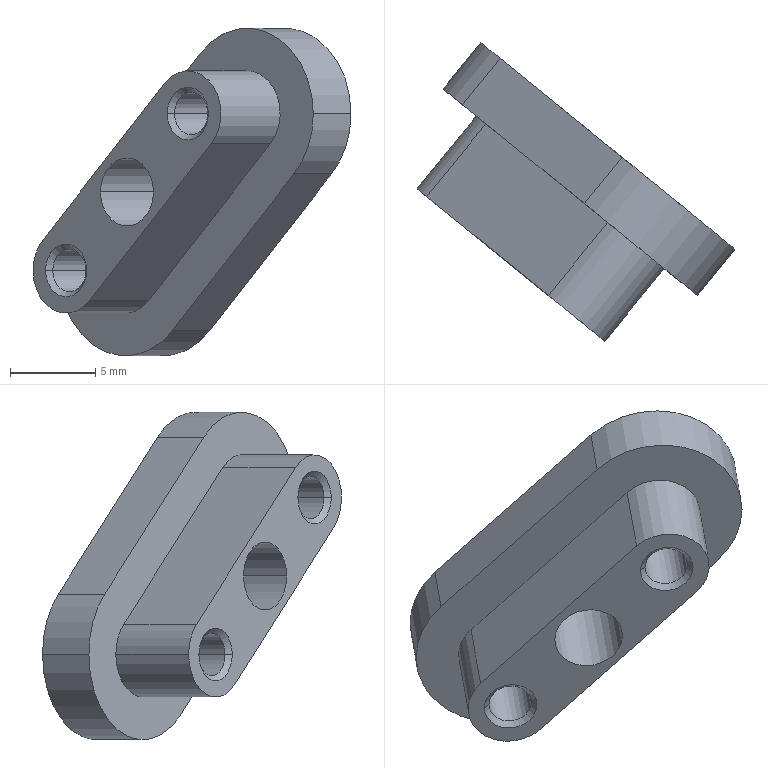Part | SolidWorks | features BaseBody 1 | 1 solid | 28 faces | box 18.629 x 17.514 x 19.192 mm | volume 992.4 mm3 | cylinder 13 | cone 8 | plane 7 | commonest cylinder face diameters 2.5 x4 10 x4 5 x3 4 x2
STEP:
#1=CARTESIAN_POINT('',(538.653,-159.567,279.158));
#2=VERTEX_POINT('',#1);
#3=CARTESIAN_POINT('',(536.714,-157.99,279.158));
#4=VERTEX_POINT('',#3);
#5=CARTESIAN_POINT('',(537.683,-158.779,279.158));
#6=DIRECTION('',(0.6309,0.7758,-0.000000012));
#7=DIRECTION('',(0.5486,-0.4461,0.7071));
#8=AXIS2_PLACEMENT_3D('',#5,#6,#7);
#9=CIRCLE('',#8,1.25);
#10=EDGE_CURVE('',#2,#4,#9,.T.);
#11=ORIENTED_EDGE('',*,*,#10,.F.);
#12=CARTESIAN_POINT('',(539.075,-159.524,279.158));
#13=VERTEX_POINT('',#12);
#14=CARTESIAN_POINT('',(539.075,-159.524,279.158));
#15=DIRECTION('',(0.9947,0.1025,-0.000000009));
#16=VECTOR('',#15,1000.);
#17=LINE('',#14,#16);
#18=EDGE_CURVE('',#2,#13,#17,.T.);
#19=ORIENTED_EDGE('',*,*,#18,.T.);
#20=CARTESIAN_POINT('',(536.67,-157.568,279.158));
#21=VERTEX_POINT('',#20);
#22=CARTESIAN_POINT('',(537.873,-158.546,279.158));
#23=DIRECTION('',(-0.6309,-0.7758,0.000000012));
#24=DIRECTION('',(-0.7758,0.6309,0.));
#25=AXIS2_PLACEMENT_3D('',#22,#23,#24);
#26=CIRCLE('',#25,1.55);
#27=EDGE_CURVE('',#21,#13,#26,.T.);
#28=ORIENTED_EDGE('',*,*,#27,.F.);
#29=CARTESIAN_POINT('',(536.67,-157.568,279.158));
#30=DIRECTION('',(-0.1025,0.9947,-0.000000009));
#31=VECTOR('',#30,1000.);
#32=LINE('',#29,#31);
#33=EDGE_CURVE('',#4,#21,#32,.T.);
#34=ORIENTED_EDGE('',*,*,#33,.F.);
#35=EDGE_LOOP('',(#11,#19,#28,#34));
#36=FACE_OUTER_BOUND('',#35,.T.);
#37=CARTESIAN_POINT('',(537.873,-158.546,279.158));
#38=DIRECTION('',(0.6309,0.7758,-0.000000012));
#39=DIRECTION('',(-0.7758,0.6309,0.));
#40=AXIS2_PLACEMENT_3D('',#37,#38,#39);
#41=CONICAL_SURFACE('',#40,1.55,0.7854);
#42=ADVANCED_FACE('',(#36),#41,.F.);
#43=CARTESIAN_POINT('',(541.752,-161.7,279.158));
#44=VERTEX_POINT('',#43);
#45=CARTESIAN_POINT('',(540.616,-160.776,275.623));
#46=VERTEX_POINT('',#45);
#47=CARTESIAN_POINT('',(537.873,-158.546,279.158));
#48=DIRECTION('',(0.6309,0.7758,-0.000000012));
#49=DIRECTION('',(0.7758,-0.6309,0.));
#50=AXIS2_PLACEMENT_3D('',#47,#48,#49);
#51=CIRCLE('',#50,5.);
#52=EDGE_CURVE('',#44,#46,#51,.T.);
#53=ORIENTED_EDGE('',*,*,#52,.F.);
#54=CARTESIAN_POINT('',(539.544,-164.416,279.158));
#55=VERTEX_POINT('',#54);
#56=CARTESIAN_POINT('',(537.493,-166.937,279.158));
#57=DIRECTION('',(-0.6309,-0.7758,0.000000012));
#58=VECTOR('',#57,1000.);
#59=LINE('',#56,#58);
#60=EDGE_CURVE('',#44,#55,#59,.T.);
#61=ORIENTED_EDGE('',*,*,#60,.T.);
#62=CARTESIAN_POINT('',(538.407,-163.492,275.623));
#63=VERTEX_POINT('',#62);
#64=CARTESIAN_POINT('',(535.664,-161.261,279.158));
#65=DIRECTION('',(0.6309,0.7758,-0.000000012));
#66=DIRECTION('',(0.7758,-0.6309,0.));
#67=AXIS2_PLACEMENT_3D('',#64,#65,#66);
#68=CIRCLE('',#67,5.);
#69=EDGE_CURVE('',#55,#63,#68,.T.);
#70=ORIENTED_EDGE('',*,*,#69,.T.);
#71=CARTESIAN_POINT('',(540.616,-160.776,275.623));
#72=DIRECTION('',(-0.6309,-0.7758,0.000000012));
#73=VECTOR('',#72,1000.);
#74=LINE('',#71,#73);
#75=EDGE_CURVE('',#46,#63,#74,.T.);
#76=ORIENTED_EDGE('',*,*,#75,.F.);
#77=EDGE_LOOP('',(#53,#61,#70,#76));
#78=FACE_OUTER_BOUND('',#77,.T.);
#79=CARTESIAN_POINT('',(533.614,-163.783,279.158));
#80=DIRECTION('',(-0.6309,-0.7758,0.000000012));
#81=DIRECTION('',(0.7758,-0.6309,0.));
#82=AXIS2_PLACEMENT_3D('',#79,#80,#81);
#83=CYLINDRICAL_SURFACE('',#82,5.);
#84=ADVANCED_FACE('',(#78),#83,.T.);
#85=CARTESIAN_POINT('',(531.276,-157.692,266.431));
#86=VERTEX_POINT('',#85);
#87=CARTESIAN_POINT('',(524.653,-152.307,269.966));
#88=VERTEX_POINT('',#87);
#89=CARTESIAN_POINT('',(528.533,-155.461,269.966));
#90=DIRECTION('',(0.6309,0.7758,-0.000000012));
#91=DIRECTION('',(-0.7758,0.6309,0.));
#92=AXIS2_PLACEMENT_3D('',#89,#90,#91);
#93=CIRCLE('',#92,5.);
#94=EDGE_CURVE('',#86,#88,#93,.T.);
#95=ORIENTED_EDGE('',*,*,#94,.T.);
#96=CARTESIAN_POINT('',(526.862,-149.591,269.966));
#97=VERTEX_POINT('',#96);
#98=CARTESIAN_POINT('',(525.442,-151.337,269.966));
#99=DIRECTION('',(0.6309,0.7758,-0.000000012));
#100=VECTOR('',#99,1000.);
#101=LINE('',#98,#100);
#102=EDGE_CURVE('',#88,#97,#101,.T.);
#103=ORIENTED_EDGE('',*,*,#102,.T.);
#104=CARTESIAN_POINT('',(533.484,-154.977,266.431));
#105=VERTEX_POINT('',#104);
#106=CARTESIAN_POINT('',(530.741,-152.746,269.966));
#107=DIRECTION('',(0.6309,0.7758,-0.000000012));
#108=DIRECTION('',(-0.7758,0.6309,0.));
#109=AXIS2_PLACEMENT_3D('',#106,#107,#108);
#110=CIRCLE('',#109,5.);
#111=EDGE_CURVE('',#105,#97,#110,.T.);
#112=ORIENTED_EDGE('',*,*,#111,.F.);
#113=CARTESIAN_POINT('',(532.064,-156.722,266.431));
#114=DIRECTION('',(-0.6309,-0.7758,0.000000012));
#115=VECTOR('',#114,1000.);
#116=LINE('',#113,#115);
#117=EDGE_CURVE('',#105,#86,#116,.T.);
#118=ORIENTED_EDGE('',*,*,#117,.T.);
#119=EDGE_LOOP('',(#95,#103,#112,#118));
#120=FACE_OUTER_BOUND('',#119,.T.);
#121=CARTESIAN_POINT('',(529.321,-154.492,269.966));
#122=DIRECTION('',(0.6309,0.7758,-0.000000012));
#123=DIRECTION('',(-0.7758,0.6309,0.));
#124=AXIS2_PLACEMENT_3D('',#121,#122,#123);
#125=CYLINDRICAL_SURFACE('',#124,5.);
#126=ADVANCED_FACE('',(#120),#125,.T.);
#127=CARTESIAN_POINT('',(531.521,-153.767,269.966));
#128=VERTEX_POINT('',#127);
#129=CARTESIAN_POINT('',(529.582,-152.19,269.966));
#130=VERTEX_POINT('',#129);
#131=CARTESIAN_POINT('',(530.552,-152.979,269.966));
#132=DIRECTION('',(0.6309,0.7758,-0.000000012));
#133=DIRECTION('',(0.5486,-0.4461,0.7071));
#134=AXIS2_PLACEMENT_3D('',#131,#132,#133);
#135=CIRCLE('',#134,1.25);
#136=EDGE_CURVE('',#128,#130,#135,.T.);
#137=ORIENTED_EDGE('',*,*,#136,.F.);
#138=CARTESIAN_POINT('',(531.943,-153.724,269.966));
#139=VERTEX_POINT('',#138);
#140=CARTESIAN_POINT('',(531.943,-153.724,269.966));
#141=DIRECTION('',(0.9947,0.1025,-0.000000009));
#142=VECTOR('',#141,1000.);
#143=LINE('',#140,#142);
#144=EDGE_CURVE('',#128,#139,#143,.T.);
#145=ORIENTED_EDGE('',*,*,#144,.T.);
#146=CARTESIAN_POINT('',(529.538,-151.768,269.966));
#147=VERTEX_POINT('',#146);
#148=CARTESIAN_POINT('',(530.741,-152.746,269.966));
#149=DIRECTION('',(-0.6309,-0.7758,0.000000012));
#150=DIRECTION('',(-0.7758,0.6309,0.));
#151=AXIS2_PLACEMENT_3D('',#148,#149,#150);
#152=CIRCLE('',#151,1.55);
#153=EDGE_CURVE('',#147,#139,#152,.T.);
#154=ORIENTED_EDGE('',*,*,#153,.F.);
#155=CARTESIAN_POINT('',(529.538,-151.768,269.966));
#156=DIRECTION('',(-0.1025,0.9947,-0.000000009));
#157=VECTOR('',#156,1000.);
#158=LINE('',#155,#157);
#159=EDGE_CURVE('',#130,#147,#158,.T.);
#160=ORIENTED_EDGE('',*,*,#159,.F.);
#161=EDGE_LOOP('',(#137,#145,#154,#160));
#162=FACE_OUTER_BOUND('',#161,.T.);
#163=CARTESIAN_POINT('',(530.741,-152.746,269.966));
#164=DIRECTION('',(0.6309,0.7758,-0.000000012));
#165=DIRECTION('',(-0.7758,0.6309,0.));
#166=AXIS2_PLACEMENT_3D('',#163,#164,#165);
#167=CONICAL_SURFACE('',#166,1.55,0.7854);
#168=ADVANCED_FACE('',(#162),#167,.F.);
#169=CARTESIAN_POINT('',(532.755,-154.384,274.562));
#170=VERTEX_POINT('',#169);
#171=CARTESIAN_POINT('',(535.858,-156.908,274.562));
#172=VERTEX_POINT('',#171);
#173=CARTESIAN_POINT('',(534.307,-155.646,274.562));
#174=DIRECTION('',(-0.6309,-0.7758,0.000000012));
#175=DIRECTION('',(0.7758,-0.6309,0.));
#176=AXIS2_PLACEMENT_3D('',#173,#174,#175);
#177=CIRCLE('',#176,2.);
#178=EDGE_CURVE('',#170,#172,#177,.T.);
#179=ORIENTED_EDGE('',*,*,#178,.F.);
#180=CARTESIAN_POINT('',(527.077,-161.367,274.562));
#181=VERTEX_POINT('',#180);
#182=CARTESIAN_POINT('',(527.077,-161.367,274.562));
#183=DIRECTION('',(-0.6309,-0.7758,0.000000012));
#184=VECTOR('',#183,1000.);
#185=LINE('',#182,#184);
#186=EDGE_CURVE('',#170,#181,#185,.T.);
#187=ORIENTED_EDGE('',*,*,#186,.T.);
#188=CARTESIAN_POINT('',(530.18,-163.89,274.562));
#189=VERTEX_POINT('',#188);
#190=CARTESIAN_POINT('',(528.628,-162.628,274.562));
#191=DIRECTION('',(0.6309,0.7758,-0.000000012));
#192=DIRECTION('',(0.7758,-0.6309,0.));
#193=AXIS2_PLACEMENT_3D('',#190,#191,#192);
#194=CIRCLE('',#193,2.);
#195=EDGE_CURVE('',#189,#181,#194,.T.);
#196=ORIENTED_EDGE('',*,*,#195,.F.);
#197=CARTESIAN_POINT('',(530.18,-163.89,274.562));
#198=DIRECTION('',(-0.6309,-0.7758,0.000000012));
#199=VECTOR('',#198,1000.);
#200=LINE('',#197,#199);
#201=EDGE_CURVE('',#172,#189,#200,.T.);
#202=ORIENTED_EDGE('',*,*,#201,.F.);
#203=EDGE_LOOP('',(#179,#187,#196,#202));
#204=FACE_OUTER_BOUND('',#203,.T.);
#205=CARTESIAN_POINT('',(528.628,-162.628,274.562));
#206=DIRECTION('',(-0.6309,-0.7758,0.000000012));
#207=DIRECTION('',(0.7758,-0.6309,0.));
#208=AXIS2_PLACEMENT_3D('',#205,#206,#207);
#209=CYLINDRICAL_SURFACE('',#208,2.);
#210=ADVANCED_FACE('',(#204),#209,.F.);
#211=CARTESIAN_POINT('',(533.353,-166.084,279.158));
#212=VERTEX_POINT('',#211);
#213=CARTESIAN_POINT('',(531.414,-164.507,279.158));
#214=VERTEX_POINT('',#213);
#215=CARTESIAN_POINT('',(532.384,-165.296,279.158));
#216=DIRECTION('',(0.6309,0.7758,-0.000000012));
#217=DIRECTION('',(-0.7758,0.6309,0.));
#218=AXIS2_PLACEMENT_3D('',#215,#216,#217);
#219=CIRCLE('',#218,1.25);
#220=EDGE_CURVE('',#212,#214,#219,.T.);
#221=ORIENTED_EDGE('',*,*,#220,.F.);
#222=CARTESIAN_POINT('',(536.003,-162.826,279.158));
#223=DIRECTION('',(0.6309,0.7758,-0.000000012));
#224=VECTOR('',#223,1000.);
#225=LINE('',#222,#224);
#226=EDGE_CURVE('',#212,#2,#225,.T.);
#227=ORIENTED_EDGE('',*,*,#226,.T.);
#228=ORIENTED_EDGE('',*,*,#10,.T.);
#229=CARTESIAN_POINT('',(534.064,-161.248,279.158));
#230=DIRECTION('',(0.6309,0.7758,-0.000000012));
#231=VECTOR('',#230,1000.);
#232=LINE('',#229,#231);
#233=EDGE_CURVE('',#214,#4,#232,.T.);
#234=ORIENTED_EDGE('',*,*,#233,.F.);
#235=EDGE_LOOP('',(#221,#227,#228,#234));
#236=FACE_OUTER_BOUND('',#235,.T.);
#237=CARTESIAN_POINT('',(535.033,-162.037,279.158));
#238=DIRECTION('',(0.6309,0.7758,-0.000000012));
#239=DIRECTION('',(-0.7758,0.6309,0.));
#240=AXIS2_PLACEMENT_3D('',#237,#238,#239);
#241=CYLINDRICAL_SURFACE('',#240,1.25);
#242=ADVANCED_FACE('',(#236),#241,.F.);
#243=CARTESIAN_POINT('',(526.222,-160.284,269.966));
#244=VERTEX_POINT('',#243);
#245=CARTESIAN_POINT('',(524.282,-158.707,269.966));
#246=VERTEX_POINT('',#245);
#247=CARTESIAN_POINT('',(525.252,-159.496,269.966));
#248=DIRECTION('',(0.6309,0.7758,-0.000000012));
#249=DIRECTION('',(-0.7758,0.6309,0.));
#250=AXIS2_PLACEMENT_3D('',#247,#248,#249);
#251=CIRCLE('',#250,1.25);
#252=EDGE_CURVE('',#244,#246,#251,.T.);
#253=ORIENTED_EDGE('',*,*,#252,.F.);
#254=CARTESIAN_POINT('',(528.871,-157.026,269.966));
#255=DIRECTION('',(0.6309,0.7758,-0.000000012));
#256=VECTOR('',#255,1000.);
#257=LINE('',#254,#256);
#258=EDGE_CURVE('',#244,#128,#257,.T.);
#259=ORIENTED_EDGE('',*,*,#258,.T.);
#260=ORIENTED_EDGE('',*,*,#136,.T.);
#261=CARTESIAN_POINT('',(526.932,-155.449,269.966));
#262=DIRECTION('',(0.6309,0.7758,-0.000000012));
#263=VECTOR('',#262,1000.);
#264=LINE('',#261,#263);
#265=EDGE_CURVE('',#246,#130,#264,.T.);
#266=ORIENTED_EDGE('',*,*,#265,.F.);
#267=EDGE_LOOP('',(#253,#259,#260,#266));
#268=FACE_OUTER_BOUND('',#267,.T.);
#269=CARTESIAN_POINT('',(527.902,-156.237,269.966));
#270=DIRECTION('',(0.6309,0.7758,-0.000000012));
#271=DIRECTION('',(-0.7758,0.6309,0.));
#272=AXIS2_PLACEMENT_3D('',#269,#270,#271);
#273=CYLINDRICAL_SURFACE('',#272,1.25);
#274=ADVANCED_FACE('',(#268),#273,.F.);
#275=ORIENTED_EDGE('',*,*,#220,.T.);
#276=CARTESIAN_POINT('',(530.992,-164.55,279.158));
#277=VERTEX_POINT('',#276);
#278=CARTESIAN_POINT('',(530.992,-164.55,279.158));
#279=DIRECTION('',(-0.9947,-0.1025,0.000000009));
#280=VECTOR('',#279,1000.);
#281=LINE('',#278,#280);
#282=EDGE_CURVE('',#214,#277,#281,.T.);
#283=ORIENTED_EDGE('',*,*,#282,.T.);
#284=CARTESIAN_POINT('',(533.397,-166.506,279.158));
#285=VERTEX_POINT('',#284);
#286=CARTESIAN_POINT('',(532.194,-165.528,279.158));
#287=DIRECTION('',(0.6309,0.7758,-0.000000012));
#288=DIRECTION('',(0.7758,-0.6309,0.));
#289=AXIS2_PLACEMENT_3D('',#286,#287,#288);
#290=CIRCLE('',#289,1.55);
#291=EDGE_CURVE('',#285,#277,#290,.T.);
#292=ORIENTED_EDGE('',*,*,#291,.F.);
#293=CARTESIAN_POINT('',(533.397,-166.506,279.158));
#294=DIRECTION('',(0.1025,-0.9947,0.000000009));
#295=VECTOR('',#294,1000.);
#296=LINE('',#293,#295);
#297=EDGE_CURVE('',#212,#285,#296,.T.);
#298=ORIENTED_EDGE('',*,*,#297,.F.);
#299=EDGE_LOOP('',(#275,#283,#292,#298));
#300=FACE_OUTER_BOUND('',#299,.T.);
#301=CARTESIAN_POINT('',(532.194,-165.528,279.158));
#302=DIRECTION('',(-0.6309,-0.7758,0.000000012));
#303=DIRECTION('',(0.7758,-0.6309,0.));
#304=AXIS2_PLACEMENT_3D('',#301,#302,#303);
#305=CONICAL_SURFACE('',#304,1.55,0.7854);
#306=ADVANCED_FACE('',(#300),#305,.F.);
#307=CARTESIAN_POINT('',(523.123,-158.151,269.966));
#308=VERTEX_POINT('',#307);
#309=CARTESIAN_POINT('',(526.434,-160.844,268.198));
#310=VERTEX_POINT('',#309);
#311=CARTESIAN_POINT('',(525.062,-159.729,269.966));
#312=DIRECTION('',(-0.6309,-0.7758,0.000000012));
#313=DIRECTION('',(-0.7758,0.6309,0.));
#314=AXIS2_PLACEMENT_3D('',#311,#312,#313);
#315=CIRCLE('',#314,2.5);
#316=EDGE_CURVE('',#308,#310,#315,.T.);
#317=ORIENTED_EDGE('',*,*,#316,.F.);
#318=CARTESIAN_POINT('',(526.593,-153.884,269.966));
#319=VERTEX_POINT('',#318);
#320=CARTESIAN_POINT('',(523.123,-158.151,269.966));
#321=DIRECTION('',(0.6309,0.7758,-0.000000012));
#322=VECTOR('',#321,1000.);
#323=LINE('',#320,#322);
#324=EDGE_CURVE('',#308,#319,#323,.T.);
#325=ORIENTED_EDGE('',*,*,#324,.T.);
#326=CARTESIAN_POINT('',(529.904,-156.577,268.198));
#327=VERTEX_POINT('',#326);
#328=CARTESIAN_POINT('',(528.533,-155.461,269.966));
#329=DIRECTION('',(-0.6309,-0.7758,0.000000012));
#330=DIRECTION('',(-0.7758,0.6309,0.));
#331=AXIS2_PLACEMENT_3D('',#328,#329,#330);
#332=CIRCLE('',#331,2.5);
#333=EDGE_CURVE('',#319,#327,#332,.T.);
#334=ORIENTED_EDGE('',*,*,#333,.T.);
#335=CARTESIAN_POINT('',(529.904,-156.577,268.198));
#336=DIRECTION('',(-0.6309,-0.7758,0.000000012));
#337=VECTOR('',#336,1000.);
#338=LINE('',#335,#337);
#339=EDGE_CURVE('',#327,#310,#338,.T.);
#340=ORIENTED_EDGE('',*,*,#339,.T.);
#341=EDGE_LOOP('',(#317,#325,#334,#340));
#342=FACE_OUTER_BOUND('',#341,.T.);
#343=CARTESIAN_POINT('',(525.062,-159.729,269.966));
#344=DIRECTION('',(0.6309,0.7758,-0.000000012));
#345=DIRECTION('',(-0.7758,0.6309,0.));
#346=AXIS2_PLACEMENT_3D('',#343,#344,#345);
#347=CYLINDRICAL_SURFACE('',#346,2.5);
#348=ADVANCED_FACE('',(#342),#347,.T.);
#349=ORIENTED_EDGE('',*,*,#252,.T.);
#350=CARTESIAN_POINT('',(523.86,-158.751,269.966));
#351=VERTEX_POINT('',#350);
#352=CARTESIAN_POINT('',(523.86,-158.751,269.966));
#353=DIRECTION('',(-0.9947,-0.1025,0.000000009));
#354=VECTOR('',#353,1000.);
#355=LINE('',#352,#354);
#356=EDGE_CURVE('',#246,#351,#355,.T.);
#357=ORIENTED_EDGE('',*,*,#356,.T.);
#358=CARTESIAN_POINT('',(526.265,-160.706,269.966));
#359=VERTEX_POINT('',#358);
#360=CARTESIAN_POINT('',(525.062,-159.729,269.966));
#361=DIRECTION('',(0.6309,0.7758,-0.000000012));
#362=DIRECTION('',(0.7758,-0.6309,0.));
#363=AXIS2_PLACEMENT_3D('',#360,#361,#362);
#364=CIRCLE('',#363,1.55);
#365=EDGE_CURVE('',#359,#351,#364,.T.);
#366=ORIENTED_EDGE('',*,*,#365,.F.);
#367=CARTESIAN_POINT('',(526.265,-160.706,269.966));
#368=DIRECTION('',(0.1025,-0.9947,0.000000009));
#369=VECTOR('',#368,1000.);
#370=LINE('',#367,#369);
#371=EDGE_CURVE('',#244,#359,#370,.T.);
#372=ORIENTED_EDGE('',*,*,#371,.F.);
#373=EDGE_LOOP('',(#349,#357,#366,#372));
#374=FACE_OUTER_BOUND('',#373,.T.);
#375=CARTESIAN_POINT('',(525.062,-159.729,269.966));
#376=DIRECTION('',(-0.6309,-0.7758,0.000000012));
#377=DIRECTION('',(0.7758,-0.6309,0.));
#378=AXIS2_PLACEMENT_3D('',#375,#376,#377);
#379=CONICAL_SURFACE('',#378,1.55,0.7854);
#380=ADVANCED_FACE('',(#374),#379,.F.);
#381=ORIENTED_EDGE('',*,*,#27,.T.);
#382=CARTESIAN_POINT('',(537.873,-158.546,279.158));
#383=DIRECTION('',(-0.6309,-0.7758,0.000000012));
#384=DIRECTION('',(-0.7758,0.6309,0.));
#385=AXIS2_PLACEMENT_3D('',#382,#383,#384);
#386=CIRCLE('',#385,1.55);
#387=EDGE_CURVE('',#13,#21,#386,.T.);
#388=ORIENTED_EDGE('',*,*,#387,.T.);
#389=EDGE_LOOP('',(#381,#388));
#390=FACE_BOUND('',#389,.T.);
#391=CARTESIAN_POINT('',(527.998,-150.515,273.502));
#392=VERTEX_POINT('',#391);
#393=CARTESIAN_POINT('',(535.13,-156.315,282.694));
#394=VERTEX_POINT('',#393);
#395=CARTESIAN_POINT('',(527.998,-150.515,273.502));
#396=DIRECTION('',(0.5486,-0.4461,0.7071));
#397=VECTOR('',#396,1000.);
#398=LINE('',#395,#397);
#399=EDGE_CURVE('',#392,#394,#398,.T.);
#400=ORIENTED_EDGE('',*,*,#399,.T.);
#401=CARTESIAN_POINT('',(537.873,-158.546,279.158));
#402=DIRECTION('',(0.6309,0.7758,-0.000000012));
#403=DIRECTION('',(0.7758,-0.6309,0.));
#404=AXIS2_PLACEMENT_3D('',#401,#402,#403);
#405=CIRCLE('',#404,5.);
#406=EDGE_CURVE('',#394,#44,#405,.T.);
#407=ORIENTED_EDGE('',*,*,#406,.T.);
#408=ORIENTED_EDGE('',*,*,#52,.T.);
#409=CARTESIAN_POINT('',(540.616,-160.776,275.623));
#410=DIRECTION('',(-0.5486,0.4461,-0.7071));
#411=VECTOR('',#410,1000.);
#412=LINE('',#409,#411);
#413=EDGE_CURVE('',#46,#105,#412,.T.);
#414=ORIENTED_EDGE('',*,*,#413,.T.);
#415=ORIENTED_EDGE('',*,*,#111,.T.);
#416=CARTESIAN_POINT('',(530.741,-152.746,269.966));
#417=DIRECTION('',(0.6309,0.7758,-0.000000012));
#418=DIRECTION('',(-0.7758,0.6309,0.));
#419=AXIS2_PLACEMENT_3D('',#416,#417,#418);
#420=CIRCLE('',#419,5.);
#421=EDGE_CURVE('',#97,#392,#420,.T.);
#422=ORIENTED_EDGE('',*,*,#421,.T.);
#423=EDGE_LOOP('',(#400,#407,#408,#414,#415,#422));
#424=FACE_OUTER_BOUND('',#423,.T.);
#425=ORIENTED_EDGE('',*,*,#153,.T.);
#426=CARTESIAN_POINT('',(530.741,-152.746,269.966));
#427=DIRECTION('',(-0.6309,-0.7758,0.000000012));
#428=DIRECTION('',(-0.7758,0.6309,0.));
#429=AXIS2_PLACEMENT_3D('',#426,#427,#428);
#430=CIRCLE('',#429,1.55);
#431=EDGE_CURVE('',#139,#147,#430,.T.);
#432=ORIENTED_EDGE('',*,*,#431,.T.);
#433=EDGE_LOOP('',(#425,#432));
#434=FACE_BOUND('',#433,.T.);
#435=CARTESIAN_POINT('',(534.307,-155.646,274.562));
#436=DIRECTION('',(-0.6309,-0.7758,0.000000012));
#437=DIRECTION('',(0.7758,-0.6309,0.));
#438=AXIS2_PLACEMENT_3D('',#435,#436,#437);
#439=CIRCLE('',#438,2.);
#440=EDGE_CURVE('',#172,#170,#439,.T.);
#441=ORIENTED_EDGE('',*,*,#440,.T.);
#442=ORIENTED_EDGE('',*,*,#178,.T.);
#443=EDGE_LOOP('',(#441,#442));
#444=FACE_BOUND('',#443,.T.);
#445=CARTESIAN_POINT('',(537.873,-158.546,286.23));
#446=DIRECTION('',(0.6309,0.7758,-0.000000012));
#447=DIRECTION('',(-0.7758,0.6309,0.));
#448=AXIS2_PLACEMENT_3D('',#445,#446,#447);
#449=PLANE('',#448);
#450=ADVANCED_FACE('',(#390,#424,#434,#444),#449,.T.);
#451=ORIENTED_EDGE('',*,*,#18,.F.);
#452=CARTESIAN_POINT('',(537.683,-158.779,279.158));
#453=DIRECTION('',(0.6309,0.7758,-0.000000012));
#454=DIRECTION('',(0.5486,-0.4461,0.7071));
#455=AXIS2_PLACEMENT_3D('',#452,#453,#454);
#456=CIRCLE('',#455,1.25);
#457=EDGE_CURVE('',#4,#2,#456,.T.);
#458=ORIENTED_EDGE('',*,*,#457,.F.);
#459=ORIENTED_EDGE('',*,*,#33,.T.);
#460=ORIENTED_EDGE('',*,*,#387,.F.);
#461=EDGE_LOOP('',(#451,#458,#459,#460));
#462=FACE_OUTER_BOUND('',#461,.T.);
#463=CARTESIAN_POINT('',(537.873,-158.546,279.158));
#464=DIRECTION('',(0.6309,0.7758,-0.000000012));
#465=DIRECTION('',(-0.7758,0.6309,0.));
#466=AXIS2_PLACEMENT_3D('',#463,#464,#465);
#467=CONICAL_SURFACE('',#466,1.55,0.7854);
#468=ADVANCED_FACE('',(#462),#467,.F.);
#469=ORIENTED_EDGE('',*,*,#60,.F.);
#470=ORIENTED_EDGE('',*,*,#406,.F.);
#471=CARTESIAN_POINT('',(532.921,-159.031,282.694));
#472=VERTEX_POINT('',#471);
#473=CARTESIAN_POINT('',(530.871,-161.552,282.694));
#474=DIRECTION('',(-0.6309,-0.7758,0.000000012));
#475=VECTOR('',#474,1000.);
#476=LINE('',#473,#475);
#477=EDGE_CURVE('',#394,#472,#476,.T.);
#478=ORIENTED_EDGE('',*,*,#477,.T.);
#479=CARTESIAN_POINT('',(535.664,-161.261,279.158));
#480=DIRECTION('',(0.6309,0.7758,-0.000000012));
#481=DIRECTION('',(0.7758,-0.6309,0.));
#482=AXIS2_PLACEMENT_3D('',#479,#480,#481);
#483=CIRCLE('',#482,5.);
#484=EDGE_CURVE('',#472,#55,#483,.T.);
#485=ORIENTED_EDGE('',*,*,#484,.T.);
#486=EDGE_LOOP('',(#469,#470,#478,#485));
#487=FACE_OUTER_BOUND('',#486,.T.);
#488=CARTESIAN_POINT('',(533.614,-163.783,279.158));
#489=DIRECTION('',(-0.6309,-0.7758,0.000000012));
#490=DIRECTION('',(0.7758,-0.6309,0.));
#491=AXIS2_PLACEMENT_3D('',#488,#489,#490);
#492=CYLINDRICAL_SURFACE('',#491,5.);
#493=ADVANCED_FACE('',(#487),#492,.T.);
#494=ORIENTED_EDGE('',*,*,#399,.F.);
#495=CARTESIAN_POINT('',(525.79,-153.231,273.502));
#496=VERTEX_POINT('',#495);
#497=CARTESIAN_POINT('',(525.79,-153.231,273.502));
#498=DIRECTION('',(0.6309,0.7758,-0.000000012));
#499=VECTOR('',#498,1000.);
#500=LINE('',#497,#499);
#501=EDGE_CURVE('',#496,#392,#500,.T.);
#502=ORIENTED_EDGE('',*,*,#501,.F.);
#503=CARTESIAN_POINT('',(532.921,-159.031,282.694));
#504=DIRECTION('',(-0.5486,0.4461,-0.7071));
#505=VECTOR('',#504,1000.);
#506=LINE('',#503,#505);
#507=EDGE_CURVE('',#472,#496,#506,.T.);
#508=ORIENTED_EDGE('',*,*,#507,.F.);
#509=ORIENTED_EDGE('',*,*,#477,.F.);
#510=EDGE_LOOP('',(#494,#502,#508,#509));
#511=FACE_OUTER_BOUND('',#510,.T.);
#512=CARTESIAN_POINT('',(528.725,-156.906,278.098));
#513=DIRECTION('',(0.5486,-0.4461,-0.7071));
#514=DIRECTION('',(-0.7901,0.,-0.613));
#515=AXIS2_PLACEMENT_3D('',#512,#513,#514);
#516=PLANE('',#515);
#517=ADVANCED_FACE('',(#511),#516,.F.);
#518=ORIENTED_EDGE('',*,*,#102,.F.);
#519=CARTESIAN_POINT('',(528.533,-155.461,269.966));
#520=DIRECTION('',(0.6309,0.7758,-0.000000012));
#521=DIRECTION('',(-0.7758,0.6309,0.));
#522=AXIS2_PLACEMENT_3D('',#519,#520,#521);
#523=CIRCLE('',#522,5.);
#524=EDGE_CURVE('',#88,#496,#523,.T.);
#525=ORIENTED_EDGE('',*,*,#524,.T.);
#526=ORIENTED_EDGE('',*,*,#501,.T.);
#527=ORIENTED_EDGE('',*,*,#421,.F.);
#528=EDGE_LOOP('',(#518,#525,#526,#527));
#529=FACE_OUTER_BOUND('',#528,.T.);
#530=CARTESIAN_POINT('',(529.321,-154.492,269.966));
#531=DIRECTION('',(0.6309,0.7758,-0.000000012));
#532=DIRECTION('',(-0.7758,0.6309,0.));
#533=AXIS2_PLACEMENT_3D('',#530,#531,#532);
#534=CYLINDRICAL_SURFACE('',#533,5.);
#535=ADVANCED_FACE('',(#529),#534,.T.);
#536=ORIENTED_EDGE('',*,*,#117,.F.);
#537=ORIENTED_EDGE('',*,*,#413,.F.);
#538=ORIENTED_EDGE('',*,*,#75,.T.);
#539=CARTESIAN_POINT('',(538.407,-163.492,275.623));
#540=DIRECTION('',(-0.5486,0.4461,-0.7071));
#541=VECTOR('',#540,1000.);
#542=LINE('',#539,#541);
#543=EDGE_CURVE('',#63,#86,#542,.T.);
#544=ORIENTED_EDGE('',*,*,#543,.T.);
#545=EDGE_LOOP('',(#536,#537,#538,#544));
#546=FACE_OUTER_BOUND('',#545,.T.);
#547=CARTESIAN_POINT('',(534.211,-161.368,271.027));
#548=DIRECTION('',(0.5486,-0.4461,-0.7071));
#549=DIRECTION('',(-0.7901,0.,-0.613));
#550=AXIS2_PLACEMENT_3D('',#547,#548,#549);
#551=PLANE('',#550);
#552=ADVANCED_FACE('',(#546),#551,.T.);
#553=ORIENTED_EDGE('',*,*,#144,.F.);
#554=CARTESIAN_POINT('',(530.552,-152.979,269.966));
#555=DIRECTION('',(0.6309,0.7758,-0.000000012));
#556=DIRECTION('',(0.5486,-0.4461,0.7071));
#557=AXIS2_PLACEMENT_3D('',#554,#555,#556);
#558=CIRCLE('',#557,1.25);
#559=EDGE_CURVE('',#130,#128,#558,.T.);
#560=ORIENTED_EDGE('',*,*,#559,.F.);
#561=ORIENTED_EDGE('',*,*,#159,.T.);
#562=ORIENTED_EDGE('',*,*,#431,.F.);
#563=EDGE_LOOP('',(#553,#560,#561,#562));
#564=FACE_OUTER_BOUND('',#563,.T.);
#565=CARTESIAN_POINT('',(530.741,-152.746,269.966));
#566=DIRECTION('',(0.6309,0.7758,-0.000000012));
#567=DIRECTION('',(-0.7758,0.6309,0.));
#568=AXIS2_PLACEMENT_3D('',#565,#566,#567);
#569=CONICAL_SURFACE('',#568,1.55,0.7854);
#570=ADVANCED_FACE('',(#564),#569,.F.);
#571=ORIENTED_EDGE('',*,*,#186,.F.);
#572=ORIENTED_EDGE('',*,*,#440,.F.);
#573=ORIENTED_EDGE('',*,*,#201,.T.);
#574=CARTESIAN_POINT('',(528.628,-162.628,274.562));
#575=DIRECTION('',(0.6309,0.7758,-0.000000012));
#576=DIRECTION('',(0.7758,-0.6309,0.));
#577=AXIS2_PLACEMENT_3D('',#574,#575,#576);
#578=CIRCLE('',#577,2.);
#579=EDGE_CURVE('',#181,#189,#578,.T.);
#580=ORIENTED_EDGE('',*,*,#579,.F.);
#581=EDGE_LOOP('',(#571,#572,#573,#580));
#582=FACE_OUTER_BOUND('',#581,.T.);
#583=CARTESIAN_POINT('',(528.628,-162.628,274.562));
#584=DIRECTION('',(-0.6309,-0.7758,0.000000012));
#585=DIRECTION('',(0.7758,-0.6309,0.));
#586=AXIS2_PLACEMENT_3D('',#583,#584,#585);
#587=CYLINDRICAL_SURFACE('',#586,2.);
#588=ADVANCED_FACE('',(#582),#587,.F.);
#589=ORIENTED_EDGE('',*,*,#226,.F.);
#590=CARTESIAN_POINT('',(532.384,-165.296,279.158));
#591=DIRECTION('',(0.6309,0.7758,-0.000000012));
#592=DIRECTION('',(-0.7758,0.6309,0.));
#593=AXIS2_PLACEMENT_3D('',#590,#591,#592);
#594=CIRCLE('',#593,1.25);
#595=EDGE_CURVE('',#214,#212,#594,.T.);
#596=ORIENTED_EDGE('',*,*,#595,.F.);
#597=ORIENTED_EDGE('',*,*,#233,.T.);
#598=ORIENTED_EDGE('',*,*,#457,.T.);
#599=EDGE_LOOP('',(#589,#596,#597,#598));
#600=FACE_OUTER_BOUND('',#599,.T.);
#601=CARTESIAN_POINT('',(535.033,-162.037,279.158));
#602=DIRECTION('',(0.6309,0.7758,-0.000000012));
#603=DIRECTION('',(-0.7758,0.6309,0.));
#604=AXIS2_PLACEMENT_3D('',#601,#602,#603);
#605=CYLINDRICAL_SURFACE('',#604,1.25);
#606=ADVANCED_FACE('',(#600),#605,.F.);
#607=CARTESIAN_POINT('',(527.161,-154.346,271.734));
#608=VERTEX_POINT('',#607);
#609=CARTESIAN_POINT('',(528.533,-155.461,269.966));
#610=DIRECTION('',(-0.6309,-0.7758,0.000000012));
#611=DIRECTION('',(-0.7758,0.6309,0.));
#612=AXIS2_PLACEMENT_3D('',#609,#610,#611);
#613=CIRCLE('',#612,2.5);
#614=EDGE_CURVE('',#608,#319,#613,.T.);
#615=ORIENTED_EDGE('',*,*,#614,.F.);
#616=CARTESIAN_POINT('',(534.293,-160.146,280.926));
#617=VERTEX_POINT('',#616);
#618=CARTESIAN_POINT('',(534.293,-160.146,280.926));
#619=DIRECTION('',(-0.5486,0.4461,-0.7071));
#620=VECTOR('',#619,1000.);
#621=LINE('',#618,#620);
#622=EDGE_CURVE('',#617,#608,#621,.T.);
#623=ORIENTED_EDGE('',*,*,#622,.F.);
#624=CARTESIAN_POINT('',(537.036,-162.377,277.391));
#625=VERTEX_POINT('',#624);
#626=CARTESIAN_POINT('',(535.664,-161.261,279.158));
#627=DIRECTION('',(-0.6309,-0.7758,0.000000012));
#628=DIRECTION('',(-0.7758,0.6309,0.));
#629=AXIS2_PLACEMENT_3D('',#626,#627,#628);
#630=CIRCLE('',#629,2.5);
#631=EDGE_CURVE('',#625,#617,#630,.T.);
#632=ORIENTED_EDGE('',*,*,#631,.F.);
#633=CARTESIAN_POINT('',(529.904,-156.577,268.198));
#634=DIRECTION('',(0.5486,-0.4461,0.7071));
#635=VECTOR('',#634,1000.);
#636=LINE('',#633,#635);
#637=EDGE_CURVE('',#327,#625,#636,.T.);
#638=ORIENTED_EDGE('',*,*,#637,.F.);
#639=ORIENTED_EDGE('',*,*,#333,.F.);
#640=EDGE_LOOP('',(#615,#623,#632,#638,#639));
#641=FACE_BOUND('',#640,.T.);
#642=ORIENTED_EDGE('',*,*,#507,.T.);
#643=ORIENTED_EDGE('',*,*,#524,.F.);
#644=ORIENTED_EDGE('',*,*,#94,.F.);
#645=ORIENTED_EDGE('',*,*,#543,.F.);
#646=ORIENTED_EDGE('',*,*,#69,.F.);
#647=ORIENTED_EDGE('',*,*,#484,.F.);
#648=EDGE_LOOP('',(#642,#643,#644,#645,#646,#647));
#649=FACE_OUTER_BOUND('',#648,.T.);
#650=CARTESIAN_POINT('',(532.098,-158.361,274.562));
#651=DIRECTION('',(0.6309,0.7758,-0.000000012));
#652=DIRECTION('',(-0.7758,0.6309,0.));
#653=AXIS2_PLACEMENT_3D('',#650,#651,#652);
#654=PLANE('',#653);
#655=ADVANCED_FACE('',(#641,#649),#654,.F.);
#656=ORIENTED_EDGE('',*,*,#258,.F.);
#657=CARTESIAN_POINT('',(525.252,-159.496,269.966));
#658=DIRECTION('',(0.6309,0.7758,-0.000000012));
#659=DIRECTION('',(-0.7758,0.6309,0.));
#660=AXIS2_PLACEMENT_3D('',#657,#658,#659);
#661=CIRCLE('',#660,1.25);
#662=EDGE_CURVE('',#246,#244,#661,.T.);
#663=ORIENTED_EDGE('',*,*,#662,.F.);
#664=ORIENTED_EDGE('',*,*,#265,.T.);
#665=ORIENTED_EDGE('',*,*,#559,.T.);
#666=EDGE_LOOP('',(#656,#663,#664,#665));
#667=FACE_OUTER_BOUND('',#666,.T.);
#668=CARTESIAN_POINT('',(527.902,-156.237,269.966));
#669=DIRECTION('',(0.6309,0.7758,-0.000000012));
#670=DIRECTION('',(-0.7758,0.6309,0.));
#671=AXIS2_PLACEMENT_3D('',#668,#669,#670);
#672=CYLINDRICAL_SURFACE('',#671,1.25);
#673=ADVANCED_FACE('',(#667),#672,.F.);
#674=ORIENTED_EDGE('',*,*,#291,.T.);
#675=CARTESIAN_POINT('',(532.194,-165.528,279.158));
#676=DIRECTION('',(0.6309,0.7758,-0.000000012));
#677=DIRECTION('',(0.7758,-0.6309,0.));
#678=AXIS2_PLACEMENT_3D('',#675,#676,#677);
#679=CIRCLE('',#678,1.55);
#680=EDGE_CURVE('',#277,#285,#679,.T.);
#681=ORIENTED_EDGE('',*,*,#680,.T.);
#682=EDGE_LOOP('',(#674,#681));
#683=FACE_BOUND('',#682,.T.);
#684=CARTESIAN_POINT('',(530.823,-164.413,280.926));
#685=VERTEX_POINT('',#684);
#686=CARTESIAN_POINT('',(523.691,-158.613,271.734));
#687=VERTEX_POINT('',#686);
#688=CARTESIAN_POINT('',(530.823,-164.413,280.926));
#689=DIRECTION('',(-0.5486,0.4461,-0.7071));
#690=VECTOR('',#689,1000.);
#691=LINE('',#688,#690);
#692=EDGE_CURVE('',#685,#687,#691,.T.);
#693=ORIENTED_EDGE('',*,*,#692,.T.);
#694=CARTESIAN_POINT('',(525.062,-159.729,269.966));
#695=DIRECTION('',(-0.6309,-0.7758,0.000000012));
#696=DIRECTION('',(-0.7758,0.6309,0.));
#697=AXIS2_PLACEMENT_3D('',#694,#695,#696);
#698=CIRCLE('',#697,2.5);
#699=EDGE_CURVE('',#687,#308,#698,.T.);
#700=ORIENTED_EDGE('',*,*,#699,.T.);
#701=ORIENTED_EDGE('',*,*,#316,.T.);
#702=CARTESIAN_POINT('',(533.566,-166.644,277.391));
#703=VERTEX_POINT('',#702);
#704=CARTESIAN_POINT('',(526.434,-160.844,268.198));
#705=DIRECTION('',(0.5486,-0.4461,0.7071));
#706=VECTOR('',#705,1000.);
#707=LINE('',#704,#706);
#708=EDGE_CURVE('',#310,#703,#707,.T.);
#709=ORIENTED_EDGE('',*,*,#708,.T.);
#710=CARTESIAN_POINT('',(532.194,-165.528,279.158));
#711=DIRECTION('',(-0.6309,-0.7758,0.000000012));
#712=DIRECTION('',(-0.7758,0.6309,0.));
#713=AXIS2_PLACEMENT_3D('',#710,#711,#712);
#714=CIRCLE('',#713,2.5);
#715=EDGE_CURVE('',#703,#685,#714,.T.);
#716=ORIENTED_EDGE('',*,*,#715,.T.);
#717=EDGE_LOOP('',(#693,#700,#701,#709,#716));
#718=FACE_OUTER_BOUND('',#717,.T.);
#719=ORIENTED_EDGE('',*,*,#365,.T.);
#720=CARTESIAN_POINT('',(525.062,-159.729,269.966));
#721=DIRECTION('',(0.6309,0.7758,-0.000000012));
#722=DIRECTION('',(0.7758,-0.6309,0.));
#723=AXIS2_PLACEMENT_3D('',#720,#721,#722);
#724=CIRCLE('',#723,1.55);
#725=EDGE_CURVE('',#351,#359,#724,.T.);
#726=ORIENTED_EDGE('',*,*,#725,.T.);
#727=EDGE_LOOP('',(#719,#726));
#728=FACE_BOUND('',#727,.T.);
#729=ORIENTED_EDGE('',*,*,#195,.T.);
#730=ORIENTED_EDGE('',*,*,#579,.T.);
#731=EDGE_LOOP('',(#729,#730));
#732=FACE_BOUND('',#731,.T.);
#733=CARTESIAN_POINT('',(519.576,-155.267,269.966));
#734=DIRECTION('',(-0.6309,-0.7758,0.000000012));
#735=DIRECTION('',(0.7758,-0.6309,0.));
#736=AXIS2_PLACEMENT_3D('',#733,#734,#735);
#737=PLANE('',#736);
#738=ADVANCED_FACE('',(#683,#718,#728,#732),#737,.T.);
#739=ORIENTED_EDGE('',*,*,#282,.F.);
#740=ORIENTED_EDGE('',*,*,#595,.T.);
#741=ORIENTED_EDGE('',*,*,#297,.T.);
#742=ORIENTED_EDGE('',*,*,#680,.F.);
#743=EDGE_LOOP('',(#739,#740,#741,#742));
#744=FACE_OUTER_BOUND('',#743,.T.);
#745=CARTESIAN_POINT('',(532.194,-165.528,279.158));
#746=DIRECTION('',(-0.6309,-0.7758,0.000000012));
#747=DIRECTION('',(0.7758,-0.6309,0.));
#748=AXIS2_PLACEMENT_3D('',#745,#746,#747);
#749=CONICAL_SURFACE('',#748,1.55,0.7854);
#750=ADVANCED_FACE('',(#744),#749,.F.);
#751=CARTESIAN_POINT('',(533.566,-166.644,277.391));
#752=DIRECTION('',(0.6309,0.7758,-0.000000012));
#753=VECTOR('',#752,1000.);
#754=LINE('',#751,#753);
#755=EDGE_CURVE('',#703,#625,#754,.T.);
#756=ORIENTED_EDGE('',*,*,#755,.F.);
#757=ORIENTED_EDGE('',*,*,#708,.F.);
#758=ORIENTED_EDGE('',*,*,#339,.F.);
#759=ORIENTED_EDGE('',*,*,#637,.T.);
#760=EDGE_LOOP('',(#756,#757,#758,#759));
#761=FACE_OUTER_BOUND('',#760,.T.);
#762=CARTESIAN_POINT('',(533.566,-166.644,277.391));
#763=DIRECTION('',(-0.5486,0.4461,0.7071));
#764=DIRECTION('',(0.7901,0.,0.613));
#765=AXIS2_PLACEMENT_3D('',#762,#763,#764);
#766=PLANE('',#765);
#767=ADVANCED_FACE('',(#761),#766,.F.);
#768=ORIENTED_EDGE('',*,*,#324,.F.);
#769=ORIENTED_EDGE('',*,*,#699,.F.);
#770=CARTESIAN_POINT('',(523.691,-158.613,271.734));
#771=DIRECTION('',(0.6309,0.7758,-0.000000012));
#772=VECTOR('',#771,1000.);
#773=LINE('',#770,#772);
#774=EDGE_CURVE('',#687,#608,#773,.T.);
#775=ORIENTED_EDGE('',*,*,#774,.T.);
#776=ORIENTED_EDGE('',*,*,#614,.T.);
#777=EDGE_LOOP('',(#768,#769,#775,#776));
#778=FACE_OUTER_BOUND('',#777,.T.);
#779=CARTESIAN_POINT('',(525.062,-159.729,269.966));
#780=DIRECTION('',(0.6309,0.7758,-0.000000012));
#781=DIRECTION('',(-0.7758,0.6309,0.));
#782=AXIS2_PLACEMENT_3D('',#779,#780,#781);
#783=CYLINDRICAL_SURFACE('',#782,2.5);
#784=ADVANCED_FACE('',(#778),#783,.T.);
#785=ORIENTED_EDGE('',*,*,#774,.F.);
#786=ORIENTED_EDGE('',*,*,#692,.F.);
#787=CARTESIAN_POINT('',(534.293,-160.146,280.926));
#788=DIRECTION('',(-0.6309,-0.7758,0.000000012));
#789=VECTOR('',#788,1000.);
#790=LINE('',#787,#789);
#791=EDGE_CURVE('',#617,#685,#790,.T.);
#792=ORIENTED_EDGE('',*,*,#791,.F.);
#793=ORIENTED_EDGE('',*,*,#622,.T.);
#794=EDGE_LOOP('',(#785,#786,#792,#793));
#795=FACE_OUTER_BOUND('',#794,.T.);
#796=CARTESIAN_POINT('',(523.691,-158.613,271.734));
#797=DIRECTION('',(0.5486,-0.4461,-0.7071));
#798=DIRECTION('',(-0.7901,0.,-0.613));
#799=AXIS2_PLACEMENT_3D('',#796,#797,#798);
#800=PLANE('',#799);
#801=ADVANCED_FACE('',(#795),#800,.F.);
#802=ORIENTED_EDGE('',*,*,#791,.T.);
#803=ORIENTED_EDGE('',*,*,#715,.F.);
#804=ORIENTED_EDGE('',*,*,#755,.T.);
#805=ORIENTED_EDGE('',*,*,#631,.T.);
#806=EDGE_LOOP('',(#802,#803,#804,#805));
#807=FACE_OUTER_BOUND('',#806,.T.);
#808=CARTESIAN_POINT('',(532.194,-165.528,279.158));
#809=DIRECTION('',(0.6309,0.7758,-0.000000012));
#810=DIRECTION('',(-0.7758,0.6309,0.));
#811=AXIS2_PLACEMENT_3D('',#808,#809,#810);
#812=CYLINDRICAL_SURFACE('',#811,2.5);
#813=ADVANCED_FACE('',(#807),#812,.T.);
#814=ORIENTED_EDGE('',*,*,#356,.F.);
#815=ORIENTED_EDGE('',*,*,#662,.T.);
#816=ORIENTED_EDGE('',*,*,#371,.T.);
#817=ORIENTED_EDGE('',*,*,#725,.F.);
#818=EDGE_LOOP('',(#814,#815,#816,#817));
#819=FACE_OUTER_BOUND('',#818,.T.);
#820=CARTESIAN_POINT('',(525.062,-159.729,269.966));
#821=DIRECTION('',(-0.6309,-0.7758,0.000000012));
#822=DIRECTION('',(0.7758,-0.6309,0.));
#823=AXIS2_PLACEMENT_3D('',#820,#821,#822);
#824=CONICAL_SURFACE('',#823,1.55,0.7854);
#825=ADVANCED_FACE('',(#819),#824,.F.);
#826=CLOSED_SHELL('',(#42,#84,#126,#168,#210,#242,#274,#306,#348,#380,#450,#468,#493,#517,#535,#552,#570,#588,#606,#655,#673,#738,#750,#767,#784,#801,#813,#825));
#827=MANIFOLD_SOLID_BREP('',#826);
#828=CARTESIAN_POINT('',(0.,0.,0.));
#829=DIRECTION('',(0.,0.,1.));
#830=DIRECTION('',(1.,0.,0.));
#831=AXIS2_PLACEMENT_3D('',#828,#829,#830);
#832=(LENGTH_UNIT()NAMED_UNIT(*)SI_UNIT(.MILLI.,.METRE.));
#833=UNCERTAINTY_MEASURE_WITH_UNIT(LENGTH_MEASURE(0.00001),#832,'','');
#834=(NAMED_UNIT(*)PLANE_ANGLE_UNIT()SI_UNIT($,.RADIAN.));
#835=(NAMED_UNIT(*)SI_UNIT($,.STERADIAN.)SOLID_ANGLE_UNIT());
#836=(GEOMETRIC_REPRESENTATION_CONTEXT(3)GLOBAL_UNCERTAINTY_ASSIGNED_CONTEXT((#833))GLOBAL_UNIT_ASSIGNED_CONTEXT((#832,#834,#835))REPRESENTATION_CONTEXT('',''));
#837=ADVANCED_BREP_SHAPE_REPRESENTATION('',(#827,#831),#836);